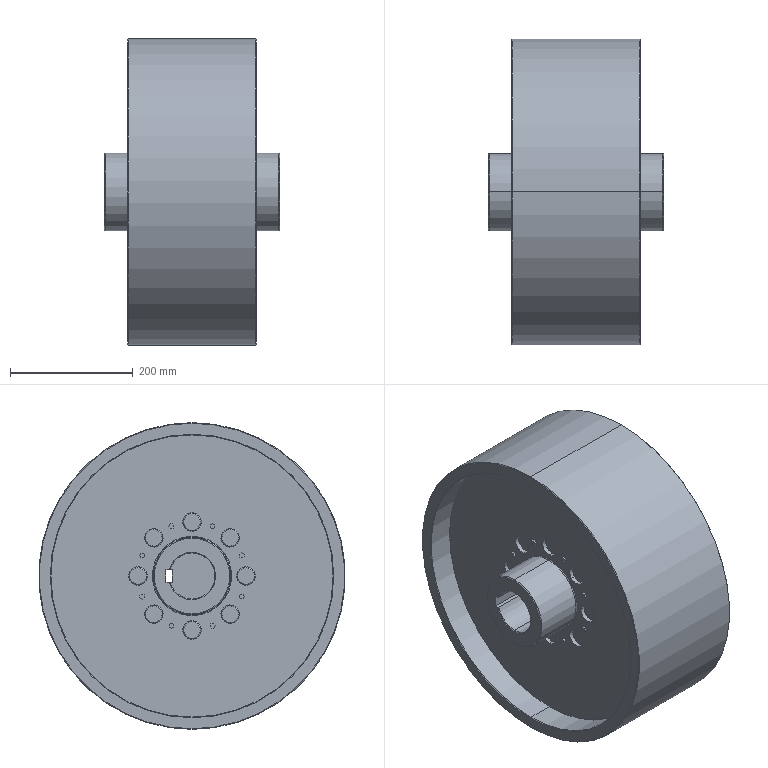Part | SolidWorks | features Chamfer 3, Fillet 2, Revolution 2, Boss 1, CirPattern 1, ICE 1, RevCut 1 | 1 solid | 203 faces | box 285.6 x 500 x 500 mm | volume 12150323 mm3 | plane 91 | cylinder 56 | cone 48 | torus 8 | commonest cylinder face diameters 30 x32 75 x6 126.5 x4 220 x4 460 x4 113.85 x2